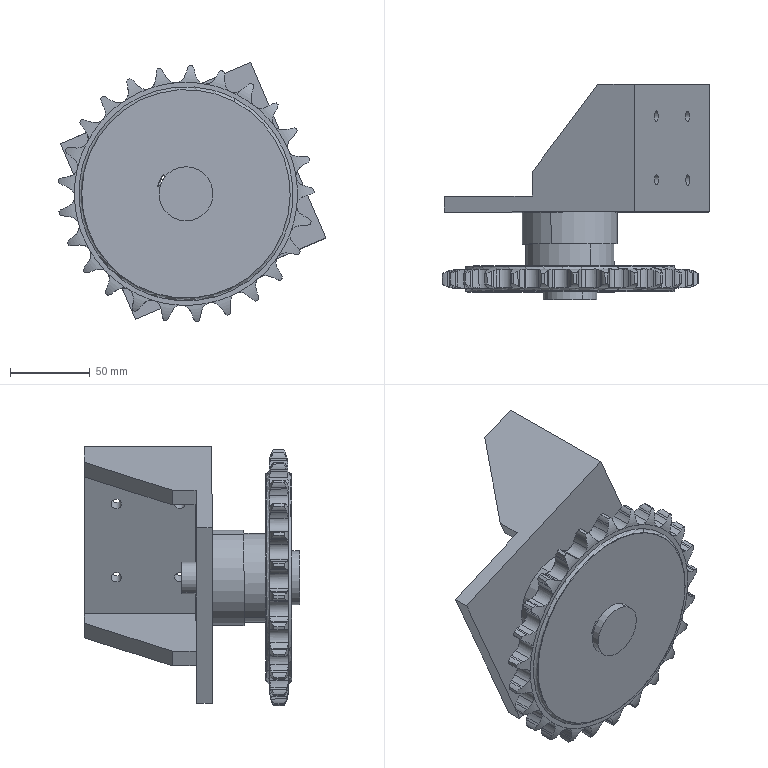Part | NX | features BREP 6 | 6 solids | 460 faces | box 168.04 x 135.33 x 162.878 mm | volume 629530 mm3 | cylinder 217 | plane 105 | torus 70 | sphere 63 | cone 5 | commonest cylinder face diameters 17.202 x53 31.126 x52 12.07 x32 161 x25 6.5 x8 46.4 x8